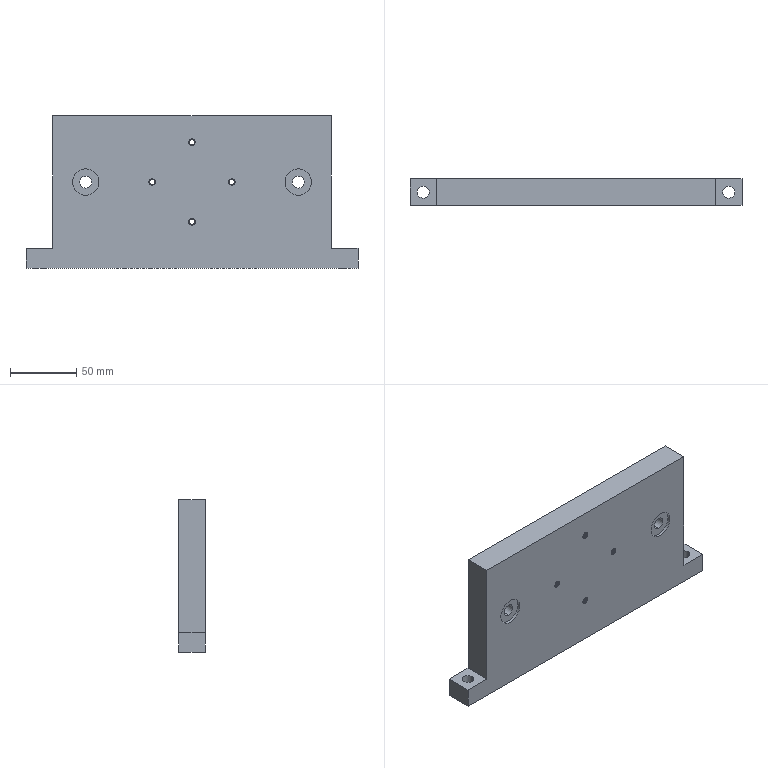Part | SolidWorks | features SweepThread 4, HoleWzd 3, Extrusion 1, ICE 1, MirrorPattern 1 | 1 solid | 278 faces | box 250 x 20 x 115 mm | volume 486183 mm3 | cylinder 244 | plane 22 | spline 12 | commonest cylinder face diameters 5 x228 9 x8 15 x4 20 x4